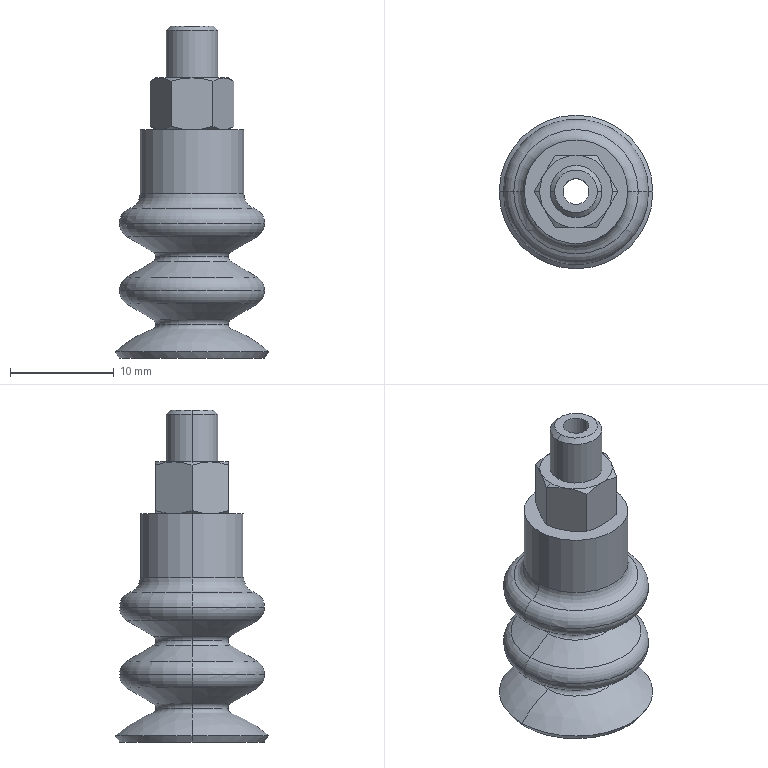Part | SolidWorks | features BaseBody 1 | 1 solid | 91 faces | box 14.806 x 14.806 x 32 mm | volume 1500 mm3 | torus 36 | cone 34 | plane 11 | cylinder 8 | sphere 2 | commonest cylinder face diameters 5 x4 2.5 x2 10 x2